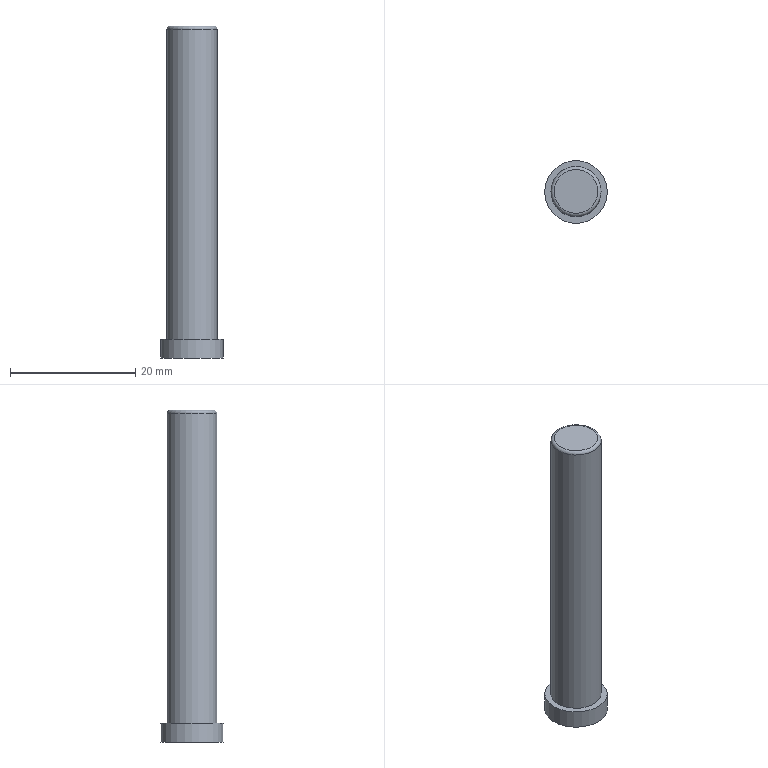Part | STEP file | lll_id4822_x_t | 1 solid | 6 faces | box 10 x 10 x 53 mm | volume 2748 mm3 | plane 3 | cylinder 2 | torus 1 | commonest cylinder face diameters 8 x1 10 x1
STEP:
#1=CARTESIAN_POINT('',(1639.5,0.00007614,10.));
#2=VERTEX_POINT('',#1);
#3=CARTESIAN_POINT('',(1643.,0.00007614,10.));
#4=DIRECTION('',(0.,0.,-1.));
#5=DIRECTION('',(-1.,0.,0.));
#6=AXIS2_PLACEMENT_3D('',#3,#4,#5);
#7=CIRCLE('',#6,3.5);
#8=EDGE_CURVE('',#2,#2,#7,.T.);
#9=ORIENTED_EDGE('',*,*,#8,.F.);
#10=EDGE_LOOP('',(#9));
#11=FACE_OUTER_BOUND('',#10,.T.);
#12=CARTESIAN_POINT('',(1643.,0.00007614,10.));
#13=DIRECTION('',(0.,0.,1.));
#14=DIRECTION('',(-1.,0.,0.));
#15=AXIS2_PLACEMENT_3D('',#12,#13,#14);
#16=PLANE('',#15);
#17=ADVANCED_FACE('',(#11),#16,.T.);
#18=CARTESIAN_POINT('',(1639.,0.00007614,-40.));
#19=VERTEX_POINT('',#18);
#20=CARTESIAN_POINT('',(1643.,0.00007614,-40.));
#21=DIRECTION('',(0.,0.,1.));
#22=DIRECTION('',(-1.,0.,0.));
#23=AXIS2_PLACEMENT_3D('',#20,#21,#22);
#24=CIRCLE('',#23,4.);
#25=EDGE_CURVE('',#19,#19,#24,.T.);
#26=ORIENTED_EDGE('',*,*,#25,.T.);
#27=EDGE_LOOP('',(#26));
#28=FACE_BOUND('',#27,.T.);
#29=CARTESIAN_POINT('',(1639.,0.00007614,9.5));
#30=VERTEX_POINT('',#29);
#31=CARTESIAN_POINT('',(1643.,0.00007614,9.5));
#32=DIRECTION('',(0.,0.,1.));
#33=DIRECTION('',(-1.,0.,0.));
#34=AXIS2_PLACEMENT_3D('',#31,#32,#33);
#35=CIRCLE('',#34,4.);
#36=EDGE_CURVE('',#30,#30,#35,.T.);
#37=ORIENTED_EDGE('',*,*,#36,.F.);
#38=EDGE_LOOP('',(#37));
#39=FACE_BOUND('',#38,.T.);
#40=CARTESIAN_POINT('',(1643.,0.00007614,-33.));
#41=DIRECTION('',(0.,0.,1.));
#42=DIRECTION('',(-1.,0.,0.));
#43=AXIS2_PLACEMENT_3D('',#40,#41,#42);
#44=CYLINDRICAL_SURFACE('',#43,4.);
#45=ADVANCED_FACE('',(#28,#39),#44,.T.);
#46=ORIENTED_EDGE('',*,*,#8,.T.);
#47=EDGE_LOOP('',(#46));
#48=FACE_BOUND('',#47,.T.);
#49=ORIENTED_EDGE('',*,*,#36,.T.);
#50=EDGE_LOOP('',(#49));
#51=FACE_BOUND('',#50,.T.);
#52=CARTESIAN_POINT('',(1643.,0.00007614,9.5));
#53=DIRECTION('',(0.,0.,1.));
#54=DIRECTION('',(-1.,0.,0.));
#55=AXIS2_PLACEMENT_3D('',#52,#53,#54);
#56=TOROIDAL_SURFACE('',#55,3.5,0.5);
#57=ADVANCED_FACE('',(#48,#51),#56,.T.);
#58=ORIENTED_EDGE('',*,*,#25,.F.);
#59=EDGE_LOOP('',(#58));
#60=FACE_BOUND('',#59,.T.);
#61=CARTESIAN_POINT('',(1638.,0.00007614,-40.));
#62=VERTEX_POINT('',#61);
#63=CARTESIAN_POINT('',(1643.,0.00007614,-40.));
#64=DIRECTION('',(0.,0.,1.));
#65=DIRECTION('',(-1.,0.,0.));
#66=AXIS2_PLACEMENT_3D('',#63,#64,#65);
#67=CIRCLE('',#66,5.);
#68=EDGE_CURVE('',#62,#62,#67,.T.);
#69=ORIENTED_EDGE('',*,*,#68,.T.);
#70=EDGE_LOOP('',(#69));
#71=FACE_BOUND('',#70,.T.);
#72=CARTESIAN_POINT('',(1643.,0.00007614,-40.));
#73=DIRECTION('',(0.,0.,1.));
#74=DIRECTION('',(-1.,0.,0.));
#75=AXIS2_PLACEMENT_3D('',#72,#73,#74);
#76=PLANE('',#75);
#77=ADVANCED_FACE('',(#60,#71),#76,.T.);
#78=ORIENTED_EDGE('',*,*,#68,.F.);
#79=EDGE_LOOP('',(#78));
#80=FACE_BOUND('',#79,.T.);
#81=CARTESIAN_POINT('',(1638.,0.00007614,-43.));
#82=VERTEX_POINT('',#81);
#83=CARTESIAN_POINT('',(1643.,0.00007614,-43.));
#84=DIRECTION('',(0.,0.,-1.));
#85=DIRECTION('',(-1.,0.,0.));
#86=AXIS2_PLACEMENT_3D('',#83,#84,#85);
#87=CIRCLE('',#86,5.);
#88=EDGE_CURVE('',#82,#82,#87,.T.);
#89=ORIENTED_EDGE('',*,*,#88,.F.);
#90=EDGE_LOOP('',(#89));
#91=FACE_BOUND('',#90,.T.);
#92=CARTESIAN_POINT('',(1643.,0.00007614,-43.));
#93=DIRECTION('',(0.,0.,1.));
#94=DIRECTION('',(-1.,0.,0.));
#95=AXIS2_PLACEMENT_3D('',#92,#93,#94);
#96=CYLINDRICAL_SURFACE('',#95,5.);
#97=ADVANCED_FACE('',(#80,#91),#96,.T.);
#98=ORIENTED_EDGE('',*,*,#88,.T.);
#99=EDGE_LOOP('',(#98));
#100=FACE_OUTER_BOUND('',#99,.T.);
#101=CARTESIAN_POINT('',(1643.,0.00007614,-43.));
#102=DIRECTION('',(0.,0.,-1.));
#103=DIRECTION('',(1.,0.,0.));
#104=AXIS2_PLACEMENT_3D('',#101,#102,#103);
#105=PLANE('',#104);
#106=ADVANCED_FACE('',(#100),#105,.T.);
#107=CLOSED_SHELL('',(#17,#45,#57,#77,#97,#106));
#108=MANIFOLD_SOLID_BREP('',#107);
#109=(LENGTH_UNIT()NAMED_UNIT(*)SI_UNIT(.MILLI.,.METRE.));
#110=UNCERTAINTY_MEASURE_WITH_UNIT(LENGTH_MEASURE(0.00002),#109,'','');
#111=(NAMED_UNIT(*)PLANE_ANGLE_UNIT()SI_UNIT($,.RADIAN.));
#112=PLANE_ANGLE_MEASURE_WITH_UNIT(PLANE_ANGLE_MEASURE(0.01745),#111);
#113=DIMENSIONAL_EXPONENTS(0.,0.,0.,0.,0.,0.,0.);
#114=(CONVERSION_BASED_UNIT('DEGREE',#112)NAMED_UNIT(#113)PLANE_ANGLE_UNIT());
#115=(NAMED_UNIT(*)SI_UNIT($,.STERADIAN.)SOLID_ANGLE_UNIT());
#116=(GEOMETRIC_REPRESENTATION_CONTEXT(3)GLOBAL_UNCERTAINTY_ASSIGNED_CONTEXT((#110))GLOBAL_UNIT_ASSIGNED_CONTEXT((#109,#114,#115))REPRESENTATION_CONTEXT('',''));
#117=ADVANCED_BREP_SHAPE_REPRESENTATION('',(#108),#116);